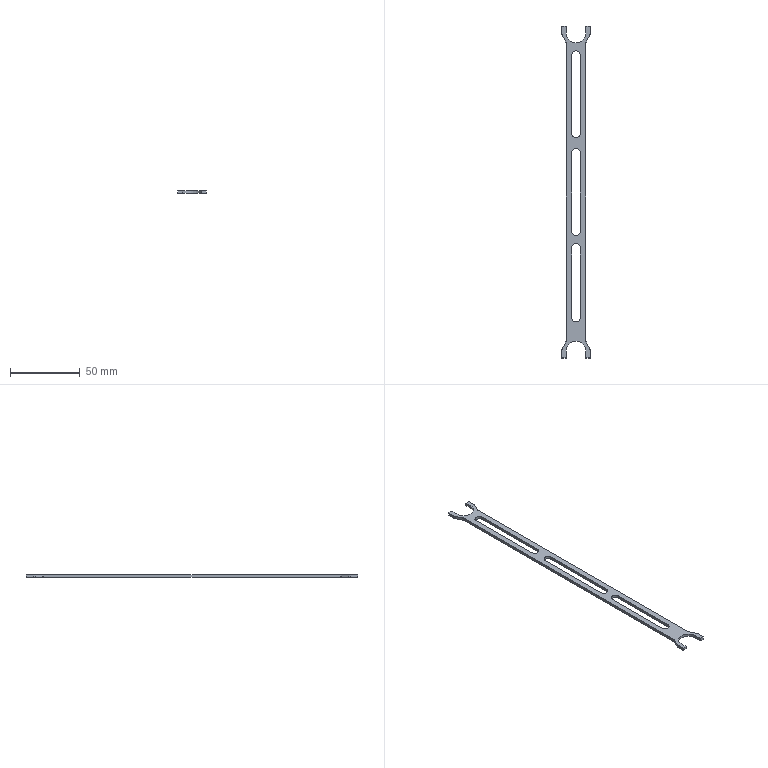Part | SolidWorks | features Extrusion 1, Fillet 1 | 1 solid | 42 faces | box 20.2 x 237.5 x 2 mm | volume 4160 mm3 | plane 26 | cylinder 16 | commonest cylinder face diameters 6 x14 14.2 x2
STEP:
#1=CARTESIAN_POINT('',(10.1,-118.75,2.));
#2=VERTEX_POINT('',#1);
#3=CARTESIAN_POINT('',(10.1,-113.469,2.));
#4=VERTEX_POINT('',#3);
#5=CARTESIAN_POINT('',(10.1,-118.75,2.));
#6=DIRECTION('',(0.,1.,0.));
#7=VECTOR('',#6,1000.);
#8=LINE('',#5,#7);
#9=EDGE_CURVE('',#2,#4,#8,.T.);
#10=ORIENTED_EDGE('',*,*,#9,.T.);
#11=CARTESIAN_POINT('',(9.774,-112.109,2.));
#12=VERTEX_POINT('',#11);
#13=CARTESIAN_POINT('',(7.1,-113.469,2.));
#14=DIRECTION('',(0.,0.,1.));
#15=DIRECTION('',(1.,0.,0.));
#16=AXIS2_PLACEMENT_3D('',#13,#14,#15);
#17=CIRCLE('',#16,3.);
#18=EDGE_CURVE('',#4,#12,#17,.T.);
#19=ORIENTED_EDGE('',*,*,#18,.T.);
#20=CARTESIAN_POINT('',(7.326,-107.291,2.));
#21=VERTEX_POINT('',#20);
#22=CARTESIAN_POINT('',(10.1,-112.75,2.));
#23=DIRECTION('',(-0.453,0.8915,0.));
#24=VECTOR('',#23,1000.);
#25=LINE('',#22,#24);
#26=EDGE_CURVE('',#12,#21,#25,.T.);
#27=ORIENTED_EDGE('',*,*,#26,.T.);
#28=CARTESIAN_POINT('',(7.,-105.931,2.));
#29=VERTEX_POINT('',#28);
#30=CARTESIAN_POINT('',(10.,-105.931,2.));
#31=DIRECTION('',(0.,0.,-1.));
#32=DIRECTION('',(1.,0.,0.));
#33=AXIS2_PLACEMENT_3D('',#30,#31,#32);
#34=CIRCLE('',#33,3.);
#35=EDGE_CURVE('',#21,#29,#34,.T.);
#36=ORIENTED_EDGE('',*,*,#35,.T.);
#37=CARTESIAN_POINT('',(7.,105.931,2.));
#38=VERTEX_POINT('',#37);
#39=CARTESIAN_POINT('',(7.,106.65,2.));
#40=DIRECTION('',(0.,1.,0.));
#41=VECTOR('',#40,1000.);
#42=LINE('',#39,#41);
#43=EDGE_CURVE('',#29,#38,#42,.T.);
#44=ORIENTED_EDGE('',*,*,#43,.T.);
#45=CARTESIAN_POINT('',(7.326,107.291,2.));
#46=VERTEX_POINT('',#45);
#47=CARTESIAN_POINT('',(10.,105.931,2.));
#48=DIRECTION('',(0.,0.,-1.));
#49=DIRECTION('',(1.,0.,0.));
#50=AXIS2_PLACEMENT_3D('',#47,#48,#49);
#51=CIRCLE('',#50,3.);
#52=EDGE_CURVE('',#38,#46,#51,.T.);
#53=ORIENTED_EDGE('',*,*,#52,.T.);
#54=CARTESIAN_POINT('',(9.774,112.109,2.));
#55=VERTEX_POINT('',#54);
#56=CARTESIAN_POINT('',(10.1,112.75,2.));
#57=DIRECTION('',(0.453,0.8915,0.));
#58=VECTOR('',#57,1000.);
#59=LINE('',#56,#58);
#60=EDGE_CURVE('',#46,#55,#59,.T.);
#61=ORIENTED_EDGE('',*,*,#60,.T.);
#62=CARTESIAN_POINT('',(10.1,113.469,2.));
#63=VERTEX_POINT('',#62);
#64=CARTESIAN_POINT('',(7.1,113.469,2.));
#65=DIRECTION('',(0.,0.,1.));
#66=DIRECTION('',(1.,0.,0.));
#67=AXIS2_PLACEMENT_3D('',#64,#65,#66);
#68=CIRCLE('',#67,3.);
#69=EDGE_CURVE('',#55,#63,#68,.T.);
#70=ORIENTED_EDGE('',*,*,#69,.T.);
#71=CARTESIAN_POINT('',(10.1,118.75,2.));
#72=VERTEX_POINT('',#71);
#73=CARTESIAN_POINT('',(10.1,118.75,2.));
#74=DIRECTION('',(0.,1.,0.));
#75=VECTOR('',#74,1000.);
#76=LINE('',#73,#75);
#77=EDGE_CURVE('',#63,#72,#76,.T.);
#78=ORIENTED_EDGE('',*,*,#77,.T.);
#79=CARTESIAN_POINT('',(7.1,118.75,2.));
#80=VERTEX_POINT('',#79);
#81=CARTESIAN_POINT('',(7.1,118.75,2.));
#82=DIRECTION('',(-1.,0.,0.));
#83=VECTOR('',#82,1000.);
#84=LINE('',#81,#83);
#85=EDGE_CURVE('',#72,#80,#84,.T.);
#86=ORIENTED_EDGE('',*,*,#85,.T.);
#87=CARTESIAN_POINT('',(7.1,113.75,2.));
#88=VERTEX_POINT('',#87);
#89=CARTESIAN_POINT('',(7.1,113.75,2.));
#90=DIRECTION('',(0.,-1.,0.));
#91=VECTOR('',#90,1000.);
#92=LINE('',#89,#91);
#93=EDGE_CURVE('',#80,#88,#92,.T.);
#94=ORIENTED_EDGE('',*,*,#93,.T.);
#95=CARTESIAN_POINT('',(-7.1,113.75,2.));
#96=VERTEX_POINT('',#95);
#97=CARTESIAN_POINT('',(0.,113.75,2.));
#98=DIRECTION('',(0.,0.,-1.));
#99=DIRECTION('',(1.,0.,0.));
#100=AXIS2_PLACEMENT_3D('',#97,#98,#99);
#101=CIRCLE('',#100,7.1);
#102=EDGE_CURVE('',#88,#96,#101,.T.);
#103=ORIENTED_EDGE('',*,*,#102,.T.);
#104=CARTESIAN_POINT('',(-7.1,118.75,2.));
#105=VERTEX_POINT('',#104);
#106=CARTESIAN_POINT('',(-7.1,113.75,2.));
#107=DIRECTION('',(0.,1.,0.));
#108=VECTOR('',#107,1000.);
#109=LINE('',#106,#108);
#110=EDGE_CURVE('',#96,#105,#109,.T.);
#111=ORIENTED_EDGE('',*,*,#110,.T.);
#112=CARTESIAN_POINT('',(-10.1,118.75,2.));
#113=VERTEX_POINT('',#112);
#114=CARTESIAN_POINT('',(-7.1,118.75,2.));
#115=DIRECTION('',(-1.,0.,0.));
#116=VECTOR('',#115,1000.);
#117=LINE('',#114,#116);
#118=EDGE_CURVE('',#105,#113,#117,.T.);
#119=ORIENTED_EDGE('',*,*,#118,.T.);
#120=CARTESIAN_POINT('',(-10.1,113.469,2.));
#121=VERTEX_POINT('',#120);
#122=CARTESIAN_POINT('',(-10.1,118.75,2.));
#123=DIRECTION('',(0.,-1.,0.));
#124=VECTOR('',#123,1000.);
#125=LINE('',#122,#124);
#126=EDGE_CURVE('',#113,#121,#125,.T.);
#127=ORIENTED_EDGE('',*,*,#126,.T.);
#128=CARTESIAN_POINT('',(-9.774,112.109,2.));
#129=VERTEX_POINT('',#128);
#130=CARTESIAN_POINT('',(-7.1,113.469,2.));
#131=DIRECTION('',(0.,0.,1.));
#132=DIRECTION('',(1.,0.,0.));
#133=AXIS2_PLACEMENT_3D('',#130,#131,#132);
#134=CIRCLE('',#133,3.);
#135=EDGE_CURVE('',#121,#129,#134,.T.);
#136=ORIENTED_EDGE('',*,*,#135,.T.);
#137=CARTESIAN_POINT('',(-7.326,107.291,2.));
#138=VERTEX_POINT('',#137);
#139=CARTESIAN_POINT('',(-10.1,112.75,2.));
#140=DIRECTION('',(0.453,-0.8915,0.));
#141=VECTOR('',#140,1000.);
#142=LINE('',#139,#141);
#143=EDGE_CURVE('',#129,#138,#142,.T.);
#144=ORIENTED_EDGE('',*,*,#143,.T.);
#145=CARTESIAN_POINT('',(-7.,105.931,2.));
#146=VERTEX_POINT('',#145);
#147=CARTESIAN_POINT('',(-10.,105.931,2.));
#148=DIRECTION('',(0.,0.,-1.));
#149=DIRECTION('',(1.,0.,0.));
#150=AXIS2_PLACEMENT_3D('',#147,#148,#149);
#151=CIRCLE('',#150,3.);
#152=EDGE_CURVE('',#138,#146,#151,.T.);
#153=ORIENTED_EDGE('',*,*,#152,.T.);
#154=CARTESIAN_POINT('',(-7.,-105.931,2.));
#155=VERTEX_POINT('',#154);
#156=CARTESIAN_POINT('',(-7.,106.65,2.));
#157=DIRECTION('',(0.,-1.,0.));
#158=VECTOR('',#157,1000.);
#159=LINE('',#156,#158);
#160=EDGE_CURVE('',#146,#155,#159,.T.);
#161=ORIENTED_EDGE('',*,*,#160,.T.);
#162=CARTESIAN_POINT('',(-7.326,-107.291,2.));
#163=VERTEX_POINT('',#162);
#164=CARTESIAN_POINT('',(-10.,-105.931,2.));
#165=DIRECTION('',(0.,0.,-1.));
#166=DIRECTION('',(1.,0.,0.));
#167=AXIS2_PLACEMENT_3D('',#164,#165,#166);
#168=CIRCLE('',#167,3.);
#169=EDGE_CURVE('',#155,#163,#168,.T.);
#170=ORIENTED_EDGE('',*,*,#169,.T.);
#171=CARTESIAN_POINT('',(-9.774,-112.109,2.));
#172=VERTEX_POINT('',#171);
#173=CARTESIAN_POINT('',(-10.1,-112.75,2.));
#174=DIRECTION('',(-0.453,-0.8915,0.));
#175=VECTOR('',#174,1000.);
#176=LINE('',#173,#175);
#177=EDGE_CURVE('',#163,#172,#176,.T.);
#178=ORIENTED_EDGE('',*,*,#177,.T.);
#179=CARTESIAN_POINT('',(-10.1,-113.469,2.));
#180=VERTEX_POINT('',#179);
#181=CARTESIAN_POINT('',(-7.1,-113.469,2.));
#182=DIRECTION('',(0.,0.,1.));
#183=DIRECTION('',(1.,0.,0.));
#184=AXIS2_PLACEMENT_3D('',#181,#182,#183);
#185=CIRCLE('',#184,3.);
#186=EDGE_CURVE('',#172,#180,#185,.T.);
#187=ORIENTED_EDGE('',*,*,#186,.T.);
#188=CARTESIAN_POINT('',(-10.1,-118.75,2.));
#189=VERTEX_POINT('',#188);
#190=CARTESIAN_POINT('',(-10.1,-118.75,2.));
#191=DIRECTION('',(0.,-1.,0.));
#192=VECTOR('',#191,1000.);
#193=LINE('',#190,#192);
#194=EDGE_CURVE('',#180,#189,#193,.T.);
#195=ORIENTED_EDGE('',*,*,#194,.T.);
#196=CARTESIAN_POINT('',(-7.1,-118.75,2.));
#197=VERTEX_POINT('',#196);
#198=CARTESIAN_POINT('',(-7.1,-118.75,2.));
#199=DIRECTION('',(1.,0.,0.));
#200=VECTOR('',#199,1000.);
#201=LINE('',#198,#200);
#202=EDGE_CURVE('',#189,#197,#201,.T.);
#203=ORIENTED_EDGE('',*,*,#202,.T.);
#204=CARTESIAN_POINT('',(-7.1,-113.75,2.));
#205=VERTEX_POINT('',#204);
#206=CARTESIAN_POINT('',(-7.1,-113.75,2.));
#207=DIRECTION('',(0.,1.,0.));
#208=VECTOR('',#207,1000.);
#209=LINE('',#206,#208);
#210=EDGE_CURVE('',#197,#205,#209,.T.);
#211=ORIENTED_EDGE('',*,*,#210,.T.);
#212=CARTESIAN_POINT('',(7.1,-113.75,2.));
#213=VERTEX_POINT('',#212);
#214=CARTESIAN_POINT('',(0.,-113.75,2.));
#215=DIRECTION('',(0.,0.,-1.));
#216=DIRECTION('',(1.,0.,0.));
#217=AXIS2_PLACEMENT_3D('',#214,#215,#216);
#218=CIRCLE('',#217,7.1);
#219=EDGE_CURVE('',#205,#213,#218,.T.);
#220=ORIENTED_EDGE('',*,*,#219,.T.);
#221=CARTESIAN_POINT('',(7.1,-118.75,2.));
#222=VERTEX_POINT('',#221);
#223=CARTESIAN_POINT('',(7.1,-113.75,2.));
#224=DIRECTION('',(0.,-1.,0.));
#225=VECTOR('',#224,1000.);
#226=LINE('',#223,#225);
#227=EDGE_CURVE('',#213,#222,#226,.T.);
#228=ORIENTED_EDGE('',*,*,#227,.T.);
#229=CARTESIAN_POINT('',(7.1,-118.75,2.));
#230=DIRECTION('',(1.,0.,0.));
#231=VECTOR('',#230,1000.);
#232=LINE('',#229,#231);
#233=EDGE_CURVE('',#222,#2,#232,.T.);
#234=ORIENTED_EDGE('',*,*,#233,.T.);
#235=EDGE_LOOP('',(#10,#19,#27,#36,#44,#53,#61,#70,#78,#86,#94,#103,#111,#119,#127,#136,#144,#153,#161,#170,#178,#187,#195,#203,#211,#220,#228,#234));
#236=FACE_OUTER_BOUND('',#235,.T.);
#237=CARTESIAN_POINT('',(-3.,98.,2.));
#238=VERTEX_POINT('',#237);
#239=CARTESIAN_POINT('',(-3.,42.,2.));
#240=VERTEX_POINT('',#239);
#241=CARTESIAN_POINT('',(-3.,98.,2.));
#242=DIRECTION('',(0.,-1.,0.));
#243=VECTOR('',#242,1000.);
#244=LINE('',#241,#243);
#245=EDGE_CURVE('',#238,#240,#244,.T.);
#246=ORIENTED_EDGE('',*,*,#245,.F.);
#247=CARTESIAN_POINT('',(3.,98.,2.));
#248=VERTEX_POINT('',#247);
#249=CARTESIAN_POINT('',(0.,98.,2.));
#250=DIRECTION('',(0.,0.,1.));
#251=DIRECTION('',(1.,0.,0.));
#252=AXIS2_PLACEMENT_3D('',#249,#250,#251);
#253=CIRCLE('',#252,3.);
#254=EDGE_CURVE('',#248,#238,#253,.T.);
#255=ORIENTED_EDGE('',*,*,#254,.F.);
#256=CARTESIAN_POINT('',(3.,42.,2.));
#257=VERTEX_POINT('',#256);
#258=CARTESIAN_POINT('',(3.,98.,2.));
#259=DIRECTION('',(0.,1.,0.));
#260=VECTOR('',#259,1000.);
#261=LINE('',#258,#260);
#262=EDGE_CURVE('',#257,#248,#261,.T.);
#263=ORIENTED_EDGE('',*,*,#262,.F.);
#264=CARTESIAN_POINT('',(0.,42.,2.));
#265=DIRECTION('',(0.,0.,1.));
#266=DIRECTION('',(1.,0.,0.));
#267=AXIS2_PLACEMENT_3D('',#264,#265,#266);
#268=CIRCLE('',#267,3.);
#269=EDGE_CURVE('',#240,#257,#268,.T.);
#270=ORIENTED_EDGE('',*,*,#269,.F.);
#271=EDGE_LOOP('',(#246,#255,#263,#270));
#272=FACE_BOUND('',#271,.T.);
#273=CARTESIAN_POINT('',(-3.,28.,2.));
#274=VERTEX_POINT('',#273);
#275=CARTESIAN_POINT('',(-3.,-28.,2.));
#276=VERTEX_POINT('',#275);
#277=CARTESIAN_POINT('',(-3.,28.,2.));
#278=DIRECTION('',(0.,-1.,0.));
#279=VECTOR('',#278,1000.);
#280=LINE('',#277,#279);
#281=EDGE_CURVE('',#274,#276,#280,.T.);
#282=ORIENTED_EDGE('',*,*,#281,.F.);
#283=CARTESIAN_POINT('',(3.,28.,2.));
#284=VERTEX_POINT('',#283);
#285=CARTESIAN_POINT('',(0.,28.,2.));
#286=DIRECTION('',(0.,0.,1.));
#287=DIRECTION('',(1.,0.,0.));
#288=AXIS2_PLACEMENT_3D('',#285,#286,#287);
#289=CIRCLE('',#288,3.);
#290=EDGE_CURVE('',#284,#274,#289,.T.);
#291=ORIENTED_EDGE('',*,*,#290,.F.);
#292=CARTESIAN_POINT('',(3.,-28.,2.));
#293=VERTEX_POINT('',#292);
#294=CARTESIAN_POINT('',(3.,28.,2.));
#295=DIRECTION('',(0.,1.,0.));
#296=VECTOR('',#295,1000.);
#297=LINE('',#294,#296);
#298=EDGE_CURVE('',#293,#284,#297,.T.);
#299=ORIENTED_EDGE('',*,*,#298,.F.);
#300=CARTESIAN_POINT('',(0.,-28.,2.));
#301=DIRECTION('',(0.,0.,1.));
#302=DIRECTION('',(1.,0.,0.));
#303=AXIS2_PLACEMENT_3D('',#300,#301,#302);
#304=CIRCLE('',#303,3.);
#305=EDGE_CURVE('',#276,#293,#304,.T.);
#306=ORIENTED_EDGE('',*,*,#305,.F.);
#307=EDGE_LOOP('',(#282,#291,#299,#306));
#308=FACE_BOUND('',#307,.T.);
#309=CARTESIAN_POINT('',(-3.,-40.,2.));
#310=VERTEX_POINT('',#309);
#311=CARTESIAN_POINT('',(-3.,-90.,2.));
#312=VERTEX_POINT('',#311);
#313=CARTESIAN_POINT('',(-3.,-40.,2.));
#314=DIRECTION('',(0.,-1.,0.));
#315=VECTOR('',#314,1000.);
#316=LINE('',#313,#315);
#317=EDGE_CURVE('',#310,#312,#316,.T.);
#318=ORIENTED_EDGE('',*,*,#317,.F.);
#319=CARTESIAN_POINT('',(3.,-40.,2.));
#320=VERTEX_POINT('',#319);
#321=CARTESIAN_POINT('',(0.,-40.,2.));
#322=DIRECTION('',(0.,0.,1.));
#323=DIRECTION('',(1.,0.,0.));
#324=AXIS2_PLACEMENT_3D('',#321,#322,#323);
#325=CIRCLE('',#324,3.);
#326=EDGE_CURVE('',#320,#310,#325,.T.);
#327=ORIENTED_EDGE('',*,*,#326,.F.);
#328=CARTESIAN_POINT('',(3.,-90.,2.));
#329=VERTEX_POINT('',#328);
#330=CARTESIAN_POINT('',(3.,-40.,2.));
#331=DIRECTION('',(0.,1.,0.));
#332=VECTOR('',#331,1000.);
#333=LINE('',#330,#332);
#334=EDGE_CURVE('',#329,#320,#333,.T.);
#335=ORIENTED_EDGE('',*,*,#334,.F.);
#336=CARTESIAN_POINT('',(0.,-90.,2.));
#337=DIRECTION('',(0.,0.,1.));
#338=DIRECTION('',(1.,0.,0.));
#339=AXIS2_PLACEMENT_3D('',#336,#337,#338);
#340=CIRCLE('',#339,3.);
#341=EDGE_CURVE('',#312,#329,#340,.T.);
#342=ORIENTED_EDGE('',*,*,#341,.F.);
#343=EDGE_LOOP('',(#318,#327,#335,#342));
#344=FACE_BOUND('',#343,.T.);
#345=CARTESIAN_POINT('',(0.,113.75,2.));
#346=DIRECTION('',(0.,0.,1.));
#347=DIRECTION('',(1.,0.,0.));
#348=AXIS2_PLACEMENT_3D('',#345,#346,#347);
#349=PLANE('',#348);
#350=ADVANCED_FACE('',(#236,#272,#308,#344),#349,.T.);
#351=CARTESIAN_POINT('',(3.,28.,0.));
#352=VERTEX_POINT('',#351);
#353=CARTESIAN_POINT('',(-3.,28.,0.));
#354=VERTEX_POINT('',#353);
#355=CARTESIAN_POINT('',(0.,28.,0.));
#356=DIRECTION('',(0.,0.,1.));
#357=DIRECTION('',(1.,0.,0.));
#358=AXIS2_PLACEMENT_3D('',#355,#356,#357);
#359=CIRCLE('',#358,3.);
#360=EDGE_CURVE('',#352,#354,#359,.T.);
#361=ORIENTED_EDGE('',*,*,#360,.T.);
#362=CARTESIAN_POINT('',(-3.,-28.,0.));
#363=VERTEX_POINT('',#362);
#364=CARTESIAN_POINT('',(-3.,28.,0.));
#365=DIRECTION('',(0.,-1.,0.));
#366=VECTOR('',#365,1000.);
#367=LINE('',#364,#366);
#368=EDGE_CURVE('',#354,#363,#367,.T.);
#369=ORIENTED_EDGE('',*,*,#368,.T.);
#370=CARTESIAN_POINT('',(3.,-28.,0.));
#371=VERTEX_POINT('',#370);
#372=CARTESIAN_POINT('',(0.,-28.,0.));
#373=DIRECTION('',(0.,0.,1.));
#374=DIRECTION('',(1.,0.,0.));
#375=AXIS2_PLACEMENT_3D('',#372,#373,#374);
#376=CIRCLE('',#375,3.);
#377=EDGE_CURVE('',#363,#371,#376,.T.);
#378=ORIENTED_EDGE('',*,*,#377,.T.);
#379=CARTESIAN_POINT('',(3.,28.,0.));
#380=DIRECTION('',(0.,1.,0.));
#381=VECTOR('',#380,1000.);
#382=LINE('',#379,#381);
#383=EDGE_CURVE('',#371,#352,#382,.T.);
#384=ORIENTED_EDGE('',*,*,#383,.T.);
#385=EDGE_LOOP('',(#361,#369,#378,#384));
#386=FACE_BOUND('',#385,.T.);
#387=CARTESIAN_POINT('',(9.774,-112.109,0.));
#388=VERTEX_POINT('',#387);
#389=CARTESIAN_POINT('',(7.326,-107.291,0.));
#390=VERTEX_POINT('',#389);
#391=CARTESIAN_POINT('',(10.1,-112.75,0.));
#392=DIRECTION('',(-0.453,0.8915,0.));
#393=VECTOR('',#392,1000.);
#394=LINE('',#391,#393);
#395=EDGE_CURVE('',#388,#390,#394,.T.);
#396=ORIENTED_EDGE('',*,*,#395,.F.);
#397=CARTESIAN_POINT('',(10.1,-113.469,0.));
#398=VERTEX_POINT('',#397);
#399=CARTESIAN_POINT('',(7.1,-113.469,0.));
#400=DIRECTION('',(0.,0.,-1.));
#401=DIRECTION('',(1.,0.,0.));
#402=AXIS2_PLACEMENT_3D('',#399,#400,#401);
#403=CIRCLE('',#402,3.);
#404=EDGE_CURVE('',#388,#398,#403,.T.);
#405=ORIENTED_EDGE('',*,*,#404,.T.);
#406=CARTESIAN_POINT('',(10.1,-118.75,0.));
#407=VERTEX_POINT('',#406);
#408=CARTESIAN_POINT('',(10.1,-118.75,0.));
#409=DIRECTION('',(0.,1.,0.));
#410=VECTOR('',#409,1000.);
#411=LINE('',#408,#410);
#412=EDGE_CURVE('',#407,#398,#411,.T.);
#413=ORIENTED_EDGE('',*,*,#412,.F.);
#414=CARTESIAN_POINT('',(7.1,-118.75,0.));
#415=VERTEX_POINT('',#414);
#416=CARTESIAN_POINT('',(7.1,-118.75,0.));
#417=DIRECTION('',(1.,0.,0.));
#418=VECTOR('',#417,1000.);
#419=LINE('',#416,#418);
#420=EDGE_CURVE('',#415,#407,#419,.T.);
#421=ORIENTED_EDGE('',*,*,#420,.F.);
#422=CARTESIAN_POINT('',(7.1,-113.75,0.));
#423=VERTEX_POINT('',#422);
#424=CARTESIAN_POINT('',(7.1,-113.75,0.));
#425=DIRECTION('',(0.,-1.,0.));
#426=VECTOR('',#425,1000.);
#427=LINE('',#424,#426);
#428=EDGE_CURVE('',#423,#415,#427,.T.);
#429=ORIENTED_EDGE('',*,*,#428,.F.);
#430=CARTESIAN_POINT('',(-7.1,-113.75,0.));
#431=VERTEX_POINT('',#430);
#432=CARTESIAN_POINT('',(0.,-113.75,0.));
#433=DIRECTION('',(0.,0.,-1.));
#434=DIRECTION('',(1.,0.,0.));
#435=AXIS2_PLACEMENT_3D('',#432,#433,#434);
#436=CIRCLE('',#435,7.1);
#437=EDGE_CURVE('',#431,#423,#436,.T.);
#438=ORIENTED_EDGE('',*,*,#437,.F.);
#439=CARTESIAN_POINT('',(-7.1,-118.75,0.));
#440=VERTEX_POINT('',#439);
#441=CARTESIAN_POINT('',(-7.1,-113.75,0.));
#442=DIRECTION('',(0.,1.,0.));
#443=VECTOR('',#442,1000.);
#444=LINE('',#441,#443);
#445=EDGE_CURVE('',#440,#431,#444,.T.);
#446=ORIENTED_EDGE('',*,*,#445,.F.);
#447=CARTESIAN_POINT('',(-10.1,-118.75,0.));
#448=VERTEX_POINT('',#447);
#449=CARTESIAN_POINT('',(-7.1,-118.75,0.));
#450=DIRECTION('',(1.,0.,0.));
#451=VECTOR('',#450,1000.);
#452=LINE('',#449,#451);
#453=EDGE_CURVE('',#448,#440,#452,.T.);
#454=ORIENTED_EDGE('',*,*,#453,.F.);
#455=CARTESIAN_POINT('',(-10.1,-113.469,0.));
#456=VERTEX_POINT('',#455);
#457=CARTESIAN_POINT('',(-10.1,-118.75,0.));
#458=DIRECTION('',(0.,-1.,0.));
#459=VECTOR('',#458,1000.);
#460=LINE('',#457,#459);
#461=EDGE_CURVE('',#456,#448,#460,.T.);
#462=ORIENTED_EDGE('',*,*,#461,.F.);
#463=CARTESIAN_POINT('',(-9.774,-112.109,0.));
#464=VERTEX_POINT('',#463);
#465=CARTESIAN_POINT('',(-7.1,-113.469,0.));
#466=DIRECTION('',(0.,0.,-1.));
#467=DIRECTION('',(1.,0.,0.));
#468=AXIS2_PLACEMENT_3D('',#465,#466,#467);
#469=CIRCLE('',#468,3.);
#470=EDGE_CURVE('',#456,#464,#469,.T.);
#471=ORIENTED_EDGE('',*,*,#470,.T.);
#472=CARTESIAN_POINT('',(-7.326,-107.291,0.));
#473=VERTEX_POINT('',#472);
#474=CARTESIAN_POINT('',(-10.1,-112.75,0.));
#475=DIRECTION('',(-0.453,-0.8915,0.));
#476=VECTOR('',#475,1000.);
#477=LINE('',#474,#476);
#478=EDGE_CURVE('',#473,#464,#477,.T.);
#479=ORIENTED_EDGE('',*,*,#478,.F.);
#480=CARTESIAN_POINT('',(-7.,-105.931,0.));
#481=VERTEX_POINT('',#480);
#482=CARTESIAN_POINT('',(-10.,-105.931,0.));
#483=DIRECTION('',(0.,0.,1.));
#484=DIRECTION('',(1.,0.,0.));
#485=AXIS2_PLACEMENT_3D('',#482,#483,#484);
#486=CIRCLE('',#485,3.);
#487=EDGE_CURVE('',#473,#481,#486,.T.);
#488=ORIENTED_EDGE('',*,*,#487,.T.);
#489=CARTESIAN_POINT('',(-7.,105.931,0.));
#490=VERTEX_POINT('',#489);
#491=CARTESIAN_POINT('',(-7.,106.65,0.));
#492=DIRECTION('',(0.,-1.,0.));
#493=VECTOR('',#492,1000.);
#494=LINE('',#491,#493);
#495=EDGE_CURVE('',#490,#481,#494,.T.);
#496=ORIENTED_EDGE('',*,*,#495,.F.);
#497=CARTESIAN_POINT('',(-7.326,107.291,0.));
#498=VERTEX_POINT('',#497);
#499=CARTESIAN_POINT('',(-10.,105.931,0.));
#500=DIRECTION('',(0.,0.,1.));
#501=DIRECTION('',(1.,0.,0.));
#502=AXIS2_PLACEMENT_3D('',#499,#500,#501);
#503=CIRCLE('',#502,3.);
#504=EDGE_CURVE('',#490,#498,#503,.T.);
#505=ORIENTED_EDGE('',*,*,#504,.T.);
#506=CARTESIAN_POINT('',(-9.774,112.109,0.));
#507=VERTEX_POINT('',#506);
#508=CARTESIAN_POINT('',(-10.1,112.75,0.));
#509=DIRECTION('',(0.453,-0.8915,0.));
#510=VECTOR('',#509,1000.);
#511=LINE('',#508,#510);
#512=EDGE_CURVE('',#507,#498,#511,.T.);
#513=ORIENTED_EDGE('',*,*,#512,.F.);
#514=CARTESIAN_POINT('',(-10.1,113.469,0.));
#515=VERTEX_POINT('',#514);
#516=CARTESIAN_POINT('',(-7.1,113.469,0.));
#517=DIRECTION('',(0.,0.,-1.));
#518=DIRECTION('',(1.,0.,0.));
#519=AXIS2_PLACEMENT_3D('',#516,#517,#518);
#520=CIRCLE('',#519,3.);
#521=EDGE_CURVE('',#507,#515,#520,.T.);
#522=ORIENTED_EDGE('',*,*,#521,.T.);
#523=CARTESIAN_POINT('',(-10.1,118.75,0.));
#524=VERTEX_POINT('',#523);
#525=CARTESIAN_POINT('',(-10.1,118.75,0.));
#526=DIRECTION('',(0.,-1.,0.));
#527=VECTOR('',#526,1000.);
#528=LINE('',#525,#527);
#529=EDGE_CURVE('',#524,#515,#528,.T.);
#530=ORIENTED_EDGE('',*,*,#529,.F.);
#531=CARTESIAN_POINT('',(-7.1,118.75,0.));
#532=VERTEX_POINT('',#531);
#533=CARTESIAN_POINT('',(-7.1,118.75,0.));
#534=DIRECTION('',(-1.,0.,0.));
#535=VECTOR('',#534,1000.);
#536=LINE('',#533,#535);
#537=EDGE_CURVE('',#532,#524,#536,.T.);
#538=ORIENTED_EDGE('',*,*,#537,.F.);
#539=CARTESIAN_POINT('',(-7.1,113.75,0.));
#540=VERTEX_POINT('',#539);
#541=CARTESIAN_POINT('',(-7.1,113.75,0.));
#542=DIRECTION('',(0.,1.,0.));
#543=VECTOR('',#542,1000.);
#544=LINE('',#541,#543);
#545=EDGE_CURVE('',#540,#532,#544,.T.);
#546=ORIENTED_EDGE('',*,*,#545,.F.);
#547=CARTESIAN_POINT('',(7.1,113.75,0.));
#548=VERTEX_POINT('',#547);
#549=CARTESIAN_POINT('',(0.,113.75,0.));
#550=DIRECTION('',(0.,0.,-1.));
#551=DIRECTION('',(1.,0.,0.));
#552=AXIS2_PLACEMENT_3D('',#549,#550,#551);
#553=CIRCLE('',#552,7.1);
#554=EDGE_CURVE('',#548,#540,#553,.T.);
#555=ORIENTED_EDGE('',*,*,#554,.F.);
#556=CARTESIAN_POINT('',(7.1,118.75,0.));
#557=VERTEX_POINT('',#556);
#558=CARTESIAN_POINT('',(7.1,113.75,0.));
#559=DIRECTION('',(0.,-1.,0.));
#560=VECTOR('',#559,1000.);
#561=LINE('',#558,#560);
#562=EDGE_CURVE('',#557,#548,#561,.T.);
#563=ORIENTED_EDGE('',*,*,#562,.F.);
#564=CARTESIAN_POINT('',(10.1,118.75,0.));
#565=VERTEX_POINT('',#564);
#566=CARTESIAN_POINT('',(7.1,118.75,0.));
#567=DIRECTION('',(-1.,0.,0.));
#568=VECTOR('',#567,1000.);
#569=LINE('',#566,#568);
#570=EDGE_CURVE('',#565,#557,#569,.T.);
#571=ORIENTED_EDGE('',*,*,#570,.F.);
#572=CARTESIAN_POINT('',(10.1,113.469,0.));
#573=VERTEX_POINT('',#572);
#574=CARTESIAN_POINT('',(10.1,118.75,0.));
#575=DIRECTION('',(0.,1.,0.));
#576=VECTOR('',#575,1000.);
#577=LINE('',#574,#576);
#578=EDGE_CURVE('',#573,#565,#577,.T.);
#579=ORIENTED_EDGE('',*,*,#578,.F.);
#580=CARTESIAN_POINT('',(9.774,112.109,0.));
#581=VERTEX_POINT('',#580);
#582=CARTESIAN_POINT('',(7.1,113.469,0.));
#583=DIRECTION('',(0.,0.,-1.));
#584=DIRECTION('',(1.,0.,0.));
#585=AXIS2_PLACEMENT_3D('',#582,#583,#584);
#586=CIRCLE('',#585,3.);
#587=EDGE_CURVE('',#573,#581,#586,.T.);
#588=ORIENTED_EDGE('',*,*,#587,.T.);
#589=CARTESIAN_POINT('',(7.326,107.291,0.));
#590=VERTEX_POINT('',#589);
#591=CARTESIAN_POINT('',(10.1,112.75,0.));
#592=DIRECTION('',(0.453,0.8915,0.));
#593=VECTOR('',#592,1000.);
#594=LINE('',#591,#593);
#595=EDGE_CURVE('',#590,#581,#594,.T.);
#596=ORIENTED_EDGE('',*,*,#595,.F.);
#597=CARTESIAN_POINT('',(7.,105.931,0.));
#598=VERTEX_POINT('',#597);
#599=CARTESIAN_POINT('',(10.,105.931,0.));
#600=DIRECTION('',(0.,0.,1.));
#601=DIRECTION('',(1.,0.,0.));
#602=AXIS2_PLACEMENT_3D('',#599,#600,#601);
#603=CIRCLE('',#602,3.);
#604=EDGE_CURVE('',#590,#598,#603,.T.);
#605=ORIENTED_EDGE('',*,*,#604,.T.);
#606=CARTESIAN_POINT('',(7.,-105.931,0.));
#607=VERTEX_POINT('',#606);
#608=CARTESIAN_POINT('',(7.,106.65,0.));
#609=DIRECTION('',(0.,1.,0.));
#610=VECTOR('',#609,1000.);
#611=LINE('',#608,#610);
#612=EDGE_CURVE('',#607,#598,#611,.T.);
#613=ORIENTED_EDGE('',*,*,#612,.F.);
#614=CARTESIAN_POINT('',(10.,-105.931,0.));
#615=DIRECTION('',(0.,0.,1.));
#616=DIRECTION('',(1.,0.,0.));
#617=AXIS2_PLACEMENT_3D('',#614,#615,#616);
#618=CIRCLE('',#617,3.);
#619=EDGE_CURVE('',#607,#390,#618,.T.);
#620=ORIENTED_EDGE('',*,*,#619,.T.);
#621=EDGE_LOOP('',(#396,#405,#413,#421,#429,#438,#446,#454,#462,#471,#479,#488,#496,#505,#513,#522,#530,#538,#546,#555,#563,#571,#579,#588,#596,#605,#613,#620));
#622=FACE_OUTER_BOUND('',#621,.T.);
#623=CARTESIAN_POINT('',(3.,98.,0.));
#624=VERTEX_POINT('',#623);
#625=CARTESIAN_POINT('',(-3.,98.,0.));
#626=VERTEX_POINT('',#625);
#627=CARTESIAN_POINT('',(0.,98.,0.));
#628=DIRECTION('',(0.,0.,1.));
#629=DIRECTION('',(1.,0.,0.));
#630=AXIS2_PLACEMENT_3D('',#627,#628,#629);
#631=CIRCLE('',#630,3.);
#632=EDGE_CURVE('',#624,#626,#631,.T.);
#633=ORIENTED_EDGE('',*,*,#632,.T.);
#634=CARTESIAN_POINT('',(-3.,42.,0.));
#635=VERTEX_POINT('',#634);
#636=CARTESIAN_POINT('',(-3.,98.,0.));
#637=DIRECTION('',(0.,-1.,0.));
#638=VECTOR('',#637,1000.);
#639=LINE('',#636,#638);
#640=EDGE_CURVE('',#626,#635,#639,.T.);
#641=ORIENTED_EDGE('',*,*,#640,.T.);
#642=CARTESIAN_POINT('',(3.,42.,0.));
#643=VERTEX_POINT('',#642);
#644=CARTESIAN_POINT('',(0.,42.,0.));
#645=DIRECTION('',(0.,0.,1.));
#646=DIRECTION('',(1.,0.,0.));
#647=AXIS2_PLACEMENT_3D('',#644,#645,#646);
#648=CIRCLE('',#647,3.);
#649=EDGE_CURVE('',#635,#643,#648,.T.);
#650=ORIENTED_EDGE('',*,*,#649,.T.);
#651=CARTESIAN_POINT('',(3.,98.,0.));
#652=DIRECTION('',(0.,1.,0.));
#653=VECTOR('',#652,1000.);
#654=LINE('',#651,#653);
#655=EDGE_CURVE('',#643,#624,#654,.T.);
#656=ORIENTED_EDGE('',*,*,#655,.T.);
#657=EDGE_LOOP('',(#633,#641,#650,#656));
#658=FACE_BOUND('',#657,.T.);
#659=CARTESIAN_POINT('',(3.,-40.,0.));
#660=VERTEX_POINT('',#659);
#661=CARTESIAN_POINT('',(-3.,-40.,0.));
#662=VERTEX_POINT('',#661);
#663=CARTESIAN_POINT('',(0.,-40.,0.));
#664=DIRECTION('',(0.,0.,1.));
#665=DIRECTION('',(1.,0.,0.));
#666=AXIS2_PLACEMENT_3D('',#663,#664,#665);
#667=CIRCLE('',#666,3.);
#668=EDGE_CURVE('',#660,#662,#667,.T.);
#669=ORIENTED_EDGE('',*,*,#668,.T.);
#670=CARTESIAN_POINT('',(-3.,-90.,0.));
#671=VERTEX_POINT('',#670);
#672=CARTESIAN_POINT('',(-3.,-40.,0.));
#673=DIRECTION('',(0.,-1.,0.));
#674=VECTOR('',#673,1000.);
#675=LINE('',#672,#674);
#676=EDGE_CURVE('',#662,#671,#675,.T.);
#677=ORIENTED_EDGE('',*,*,#676,.T.);
#678=CARTESIAN_POINT('',(3.,-90.,0.));
#679=VERTEX_POINT('',#678);
#680=CARTESIAN_POINT('',(0.,-90.,0.));
#681=DIRECTION('',(0.,0.,1.));
#682=DIRECTION('',(1.,0.,0.));
#683=AXIS2_PLACEMENT_3D('',#680,#681,#682);
#684=CIRCLE('',#683,3.);
#685=EDGE_CURVE('',#671,#679,#684,.T.);
#686=ORIENTED_EDGE('',*,*,#685,.T.);
#687=CARTESIAN_POINT('',(3.,-40.,0.));
#688=DIRECTION('',(0.,1.,0.));
#689=VECTOR('',#688,1000.);
#690=LINE('',#687,#689);
#691=EDGE_CURVE('',#679,#660,#690,.T.);
#692=ORIENTED_EDGE('',*,*,#691,.T.);
#693=EDGE_LOOP('',(#669,#677,#686,#692));
#694=FACE_BOUND('',#693,.T.);
#695=CARTESIAN_POINT('',(0.,113.75,0.));
#696=DIRECTION('',(0.,0.,1.));
#697=DIRECTION('',(1.,0.,0.));
#698=AXIS2_PLACEMENT_3D('',#695,#696,#697);
#699=PLANE('',#698);
#700=ADVANCED_FACE('',(#386,#622,#658,#694),#699,.F.);
#701=ORIENTED_EDGE('',*,*,#554,.T.);
#702=CARTESIAN_POINT('',(-7.1,113.75,2.));
#703=DIRECTION('',(0.,0.,-1.));
#704=VECTOR('',#703,1000.);
#705=LINE('',#702,#704);
#706=EDGE_CURVE('',#96,#540,#705,.T.);
#707=ORIENTED_EDGE('',*,*,#706,.F.);
#708=ORIENTED_EDGE('',*,*,#102,.F.);
#709=CARTESIAN_POINT('',(7.1,113.75,2.));
#710=DIRECTION('',(0.,0.,-1.));
#711=VECTOR('',#710,1000.);
#712=LINE('',#709,#711);
#713=EDGE_CURVE('',#88,#548,#712,.T.);
#714=ORIENTED_EDGE('',*,*,#713,.T.);
#715=EDGE_LOOP('',(#701,#707,#708,#714));
#716=FACE_OUTER_BOUND('',#715,.T.);
#717=CARTESIAN_POINT('',(0.,113.75,2.));
#718=DIRECTION('',(0.,0.,-1.));
#719=DIRECTION('',(-1.,0.,0.));
#720=AXIS2_PLACEMENT_3D('',#717,#718,#719);
#721=CYLINDRICAL_SURFACE('',#720,7.1);
#722=ADVANCED_FACE('',(#716),#721,.F.);
#723=ORIENTED_EDGE('',*,*,#545,.T.);
#724=CARTESIAN_POINT('',(-7.1,118.75,2.));
#725=DIRECTION('',(0.,0.,-1.));
#726=VECTOR('',#725,1000.);
#727=LINE('',#724,#726);
#728=EDGE_CURVE('',#105,#532,#727,.T.);
#729=ORIENTED_EDGE('',*,*,#728,.F.);
#730=ORIENTED_EDGE('',*,*,#110,.F.);
#731=ORIENTED_EDGE('',*,*,#706,.T.);
#732=EDGE_LOOP('',(#723,#729,#730,#731));
#733=FACE_OUTER_BOUND('',#732,.T.);
#734=CARTESIAN_POINT('',(-7.1,113.75,2.));
#735=DIRECTION('',(-1.,0.,0.));
#736=DIRECTION('',(0.,-1.,0.));
#737=AXIS2_PLACEMENT_3D('',#734,#735,#736);
#738=PLANE('',#737);
#739=ADVANCED_FACE('',(#733),#738,.F.);
#740=ORIENTED_EDGE('',*,*,#537,.T.);
#741=CARTESIAN_POINT('',(-10.1,118.75,2.));
#742=DIRECTION('',(0.,0.,-1.));
#743=VECTOR('',#742,1000.);
#744=LINE('',#741,#743);
#745=EDGE_CURVE('',#113,#524,#744,.T.);
#746=ORIENTED_EDGE('',*,*,#745,.F.);
#747=ORIENTED_EDGE('',*,*,#118,.F.);
#748=ORIENTED_EDGE('',*,*,#728,.T.);
#749=EDGE_LOOP('',(#740,#746,#747,#748));
#750=FACE_OUTER_BOUND('',#749,.T.);
#751=CARTESIAN_POINT('',(-7.1,118.75,2.));
#752=DIRECTION('',(0.,-1.,0.));
#753=DIRECTION('',(0.,0.,-1.));
#754=AXIS2_PLACEMENT_3D('',#751,#752,#753);
#755=PLANE('',#754);
#756=ADVANCED_FACE('',(#750),#755,.F.);
#757=ORIENTED_EDGE('',*,*,#529,.T.);
#758=CARTESIAN_POINT('',(-10.1,113.469,2.));
#759=DIRECTION('',(0.,0.,1.));
#760=VECTOR('',#759,1000.);
#761=LINE('',#758,#760);
#762=EDGE_CURVE('',#515,#121,#761,.T.);
#763=ORIENTED_EDGE('',*,*,#762,.T.);
#764=ORIENTED_EDGE('',*,*,#126,.F.);
#765=ORIENTED_EDGE('',*,*,#745,.T.);
#766=EDGE_LOOP('',(#757,#763,#764,#765));
#767=FACE_OUTER_BOUND('',#766,.T.);
#768=CARTESIAN_POINT('',(-10.1,118.75,2.));
#769=DIRECTION('',(1.,0.,0.));
#770=DIRECTION('',(0.,1.,0.));
#771=AXIS2_PLACEMENT_3D('',#768,#769,#770);
#772=PLANE('',#771);
#773=ADVANCED_FACE('',(#767),#772,.F.);
#774=ORIENTED_EDGE('',*,*,#512,.T.);
#775=CARTESIAN_POINT('',(-7.326,107.291,2.));
#776=DIRECTION('',(0.,0.,1.));
#777=VECTOR('',#776,1000.);
#778=LINE('',#775,#777);
#779=EDGE_CURVE('',#498,#138,#778,.T.);
#780=ORIENTED_EDGE('',*,*,#779,.T.);
#781=ORIENTED_EDGE('',*,*,#143,.F.);
#782=CARTESIAN_POINT('',(-9.774,112.109,2.));
#783=DIRECTION('',(0.,0.,-1.));
#784=VECTOR('',#783,1000.);
#785=LINE('',#782,#784);
#786=EDGE_CURVE('',#129,#507,#785,.T.);
#787=ORIENTED_EDGE('',*,*,#786,.T.);
#788=EDGE_LOOP('',(#774,#780,#781,#787));
#789=FACE_OUTER_BOUND('',#788,.T.);
#790=CARTESIAN_POINT('',(-10.1,112.75,2.));
#791=DIRECTION('',(0.8915,0.453,0.));
#792=DIRECTION('',(-0.453,0.8915,0.));
#793=AXIS2_PLACEMENT_3D('',#790,#791,#792);
#794=PLANE('',#793);
#795=ADVANCED_FACE('',(#789),#794,.F.);
#796=ORIENTED_EDGE('',*,*,#495,.T.);
#797=CARTESIAN_POINT('',(-7.,-105.931,2.));
#798=DIRECTION('',(0.,0.,1.));
#799=VECTOR('',#798,1000.);
#800=LINE('',#797,#799);
#801=EDGE_CURVE('',#481,#155,#800,.T.);
#802=ORIENTED_EDGE('',*,*,#801,.T.);
#803=ORIENTED_EDGE('',*,*,#160,.F.);
#804=CARTESIAN_POINT('',(-7.,105.931,0.));
#805=DIRECTION('',(0.,0.,-1.));
#806=VECTOR('',#805,1000.);
#807=LINE('',#804,#806);
#808=EDGE_CURVE('',#146,#490,#807,.T.);
#809=ORIENTED_EDGE('',*,*,#808,.T.);
#810=EDGE_LOOP('',(#796,#802,#803,#809));
#811=FACE_OUTER_BOUND('',#810,.T.);
#812=CARTESIAN_POINT('',(-7.,106.65,2.));
#813=DIRECTION('',(1.,0.,0.));
#814=DIRECTION('',(0.,0.,-1.));
#815=AXIS2_PLACEMENT_3D('',#812,#813,#814);
#816=PLANE('',#815);
#817=ADVANCED_FACE('',(#811),#816,.F.);
#818=ORIENTED_EDGE('',*,*,#478,.T.);
#819=CARTESIAN_POINT('',(-9.774,-112.109,2.));
#820=DIRECTION('',(0.,0.,1.));
#821=VECTOR('',#820,1000.);
#822=LINE('',#819,#821);
#823=EDGE_CURVE('',#464,#172,#822,.T.);
#824=ORIENTED_EDGE('',*,*,#823,.T.);
#825=ORIENTED_EDGE('',*,*,#177,.F.);
#826=CARTESIAN_POINT('',(-7.326,-107.291,0.));
#827=DIRECTION('',(0.,0.,-1.));
#828=VECTOR('',#827,1000.);
#829=LINE('',#826,#828);
#830=EDGE_CURVE('',#163,#473,#829,.T.);
#831=ORIENTED_EDGE('',*,*,#830,.T.);
#832=EDGE_LOOP('',(#818,#824,#825,#831));
#833=FACE_OUTER_BOUND('',#832,.T.);
#834=CARTESIAN_POINT('',(-10.1,-112.75,2.));
#835=DIRECTION('',(0.8915,-0.453,0.));
#836=DIRECTION('',(0.453,0.8915,0.));
#837=AXIS2_PLACEMENT_3D('',#834,#835,#836);
#838=PLANE('',#837);
#839=ADVANCED_FACE('',(#833),#838,.F.);
#840=ORIENTED_EDGE('',*,*,#194,.F.);
#841=CARTESIAN_POINT('',(-10.1,-113.469,2.));
#842=DIRECTION('',(0.,0.,-1.));
#843=VECTOR('',#842,1000.);
#844=LINE('',#841,#843);
#845=EDGE_CURVE('',#180,#456,#844,.T.);
#846=ORIENTED_EDGE('',*,*,#845,.T.);
#847=ORIENTED_EDGE('',*,*,#461,.T.);
#848=CARTESIAN_POINT('',(-10.1,-118.75,2.));
#849=DIRECTION('',(0.,0.,-1.));
#850=VECTOR('',#849,1000.);
#851=LINE('',#848,#850);
#852=EDGE_CURVE('',#189,#448,#851,.T.);
#853=ORIENTED_EDGE('',*,*,#852,.F.);
#854=EDGE_LOOP('',(#840,#846,#847,#853));
#855=FACE_OUTER_BOUND('',#854,.T.);
#856=CARTESIAN_POINT('',(-10.1,-118.75,2.));
#857=DIRECTION('',(1.,0.,0.));
#858=DIRECTION('',(0.,1.,0.));
#859=AXIS2_PLACEMENT_3D('',#856,#857,#858);
#860=PLANE('',#859);
#861=ADVANCED_FACE('',(#855),#860,.F.);
#862=ORIENTED_EDGE('',*,*,#453,.T.);
#863=CARTESIAN_POINT('',(-7.1,-118.75,2.));
#864=DIRECTION('',(0.,0.,-1.));
#865=VECTOR('',#864,1000.);
#866=LINE('',#863,#865);
#867=EDGE_CURVE('',#197,#440,#866,.T.);
#868=ORIENTED_EDGE('',*,*,#867,.F.);
#869=ORIENTED_EDGE('',*,*,#202,.F.);
#870=ORIENTED_EDGE('',*,*,#852,.T.);
#871=EDGE_LOOP('',(#862,#868,#869,#870));
#872=FACE_OUTER_BOUND('',#871,.T.);
#873=CARTESIAN_POINT('',(-7.1,-118.75,2.));
#874=DIRECTION('',(0.,1.,0.));
#875=DIRECTION('',(0.,0.,1.));
#876=AXIS2_PLACEMENT_3D('',#873,#874,#875);
#877=PLANE('',#876);
#878=ADVANCED_FACE('',(#872),#877,.F.);
#879=ORIENTED_EDGE('',*,*,#445,.T.);
#880=CARTESIAN_POINT('',(-7.1,-113.75,2.));
#881=DIRECTION('',(0.,0.,-1.));
#882=VECTOR('',#881,1000.);
#883=LINE('',#880,#882);
#884=EDGE_CURVE('',#205,#431,#883,.T.);
#885=ORIENTED_EDGE('',*,*,#884,.F.);
#886=ORIENTED_EDGE('',*,*,#210,.F.);
#887=ORIENTED_EDGE('',*,*,#867,.T.);
#888=EDGE_LOOP('',(#879,#885,#886,#887));
#889=FACE_OUTER_BOUND('',#888,.T.);
#890=CARTESIAN_POINT('',(-7.1,-113.75,2.));
#891=DIRECTION('',(-1.,0.,0.));
#892=DIRECTION('',(0.,-1.,0.));
#893=AXIS2_PLACEMENT_3D('',#890,#891,#892);
#894=PLANE('',#893);
#895=ADVANCED_FACE('',(#889),#894,.F.);
#896=ORIENTED_EDGE('',*,*,#437,.T.);
#897=CARTESIAN_POINT('',(7.1,-113.75,2.));
#898=DIRECTION('',(0.,0.,-1.));
#899=VECTOR('',#898,1000.);
#900=LINE('',#897,#899);
#901=EDGE_CURVE('',#213,#423,#900,.T.);
#902=ORIENTED_EDGE('',*,*,#901,.F.);
#903=ORIENTED_EDGE('',*,*,#219,.F.);
#904=ORIENTED_EDGE('',*,*,#884,.T.);
#905=EDGE_LOOP('',(#896,#902,#903,#904));
#906=FACE_OUTER_BOUND('',#905,.T.);
#907=CARTESIAN_POINT('',(0.,-113.75,2.));
#908=DIRECTION('',(0.,0.,-1.));
#909=DIRECTION('',(-1.,0.,0.));
#910=AXIS2_PLACEMENT_3D('',#907,#908,#909);
#911=CYLINDRICAL_SURFACE('',#910,7.1);
#912=ADVANCED_FACE('',(#906),#911,.F.);
#913=ORIENTED_EDGE('',*,*,#428,.T.);
#914=CARTESIAN_POINT('',(7.1,-118.75,2.));
#915=DIRECTION('',(0.,0.,-1.));
#916=VECTOR('',#915,1000.);
#917=LINE('',#914,#916);
#918=EDGE_CURVE('',#222,#415,#917,.T.);
#919=ORIENTED_EDGE('',*,*,#918,.F.);
#920=ORIENTED_EDGE('',*,*,#227,.F.);
#921=ORIENTED_EDGE('',*,*,#901,.T.);
#922=EDGE_LOOP('',(#913,#919,#920,#921));
#923=FACE_OUTER_BOUND('',#922,.T.);
#924=CARTESIAN_POINT('',(7.1,-113.75,2.));
#925=DIRECTION('',(1.,0.,0.));
#926=DIRECTION('',(0.,1.,0.));
#927=AXIS2_PLACEMENT_3D('',#924,#925,#926);
#928=PLANE('',#927);
#929=ADVANCED_FACE('',(#923),#928,.F.);
#930=ORIENTED_EDGE('',*,*,#420,.T.);
#931=CARTESIAN_POINT('',(10.1,-118.75,2.));
#932=DIRECTION('',(0.,0.,-1.));
#933=VECTOR('',#932,1000.);
#934=LINE('',#931,#933);
#935=EDGE_CURVE('',#2,#407,#934,.T.);
#936=ORIENTED_EDGE('',*,*,#935,.F.);
#937=ORIENTED_EDGE('',*,*,#233,.F.);
#938=ORIENTED_EDGE('',*,*,#918,.T.);
#939=EDGE_LOOP('',(#930,#936,#937,#938));
#940=FACE_OUTER_BOUND('',#939,.T.);
#941=CARTESIAN_POINT('',(7.1,-118.75,2.));
#942=DIRECTION('',(0.,1.,0.));
#943=DIRECTION('',(0.,0.,1.));
#944=AXIS2_PLACEMENT_3D('',#941,#942,#943);
#945=PLANE('',#944);
#946=ADVANCED_FACE('',(#940),#945,.F.);
#947=ORIENTED_EDGE('',*,*,#412,.T.);
#948=CARTESIAN_POINT('',(10.1,-113.469,2.));
#949=DIRECTION('',(0.,0.,1.));
#950=VECTOR('',#949,1000.);
#951=LINE('',#948,#950);
#952=EDGE_CURVE('',#398,#4,#951,.T.);
#953=ORIENTED_EDGE('',*,*,#952,.T.);
#954=ORIENTED_EDGE('',*,*,#9,.F.);
#955=ORIENTED_EDGE('',*,*,#935,.T.);
#956=EDGE_LOOP('',(#947,#953,#954,#955));
#957=FACE_OUTER_BOUND('',#956,.T.);
#958=CARTESIAN_POINT('',(10.1,-118.75,2.));
#959=DIRECTION('',(-1.,0.,0.));
#960=DIRECTION('',(0.,-1.,0.));
#961=AXIS2_PLACEMENT_3D('',#958,#959,#960);
#962=PLANE('',#961);
#963=ADVANCED_FACE('',(#957),#962,.F.);
#964=ORIENTED_EDGE('',*,*,#395,.T.);
#965=CARTESIAN_POINT('',(7.326,-107.291,2.));
#966=DIRECTION('',(0.,0.,1.));
#967=VECTOR('',#966,1000.);
#968=LINE('',#965,#967);
#969=EDGE_CURVE('',#390,#21,#968,.T.);
#970=ORIENTED_EDGE('',*,*,#969,.T.);
#971=ORIENTED_EDGE('',*,*,#26,.F.);
#972=CARTESIAN_POINT('',(9.774,-112.109,2.));
#973=DIRECTION('',(0.,0.,-1.));
#974=VECTOR('',#973,1000.);
#975=LINE('',#972,#974);
#976=EDGE_CURVE('',#12,#388,#975,.T.);
#977=ORIENTED_EDGE('',*,*,#976,.T.);
#978=EDGE_LOOP('',(#964,#970,#971,#977));
#979=FACE_OUTER_BOUND('',#978,.T.);
#980=CARTESIAN_POINT('',(10.1,-112.75,2.));
#981=DIRECTION('',(-0.8915,-0.453,0.));
#982=DIRECTION('',(0.453,-0.8915,0.));
#983=AXIS2_PLACEMENT_3D('',#980,#981,#982);
#984=PLANE('',#983);
#985=ADVANCED_FACE('',(#979),#984,.F.);
#986=ORIENTED_EDGE('',*,*,#43,.F.);
#987=CARTESIAN_POINT('',(7.,-105.931,0.));
#988=DIRECTION('',(0.,0.,-1.));
#989=VECTOR('',#988,1000.);
#990=LINE('',#987,#989);
#991=EDGE_CURVE('',#29,#607,#990,.T.);
#992=ORIENTED_EDGE('',*,*,#991,.T.);
#993=ORIENTED_EDGE('',*,*,#612,.T.);
#994=CARTESIAN_POINT('',(7.,105.931,2.));
#995=DIRECTION('',(0.,0.,1.));
#996=VECTOR('',#995,1000.);
#997=LINE('',#994,#996);
#998=EDGE_CURVE('',#598,#38,#997,.T.);
#999=ORIENTED_EDGE('',*,*,#998,.T.);
#1000=EDGE_LOOP('',(#986,#992,#993,#999));
#1001=FACE_OUTER_BOUND('',#1000,.T.);
#1002=CARTESIAN_POINT('',(7.,106.65,2.));
#1003=DIRECTION('',(-1.,0.,0.));
#1004=DIRECTION('',(0.,0.,1.));
#1005=AXIS2_PLACEMENT_3D('',#1002,#1003,#1004);
#1006=PLANE('',#1005);
#1007=ADVANCED_FACE('',(#1001),#1006,.F.);
#1008=ORIENTED_EDGE('',*,*,#595,.T.);
#1009=CARTESIAN_POINT('',(9.774,112.109,2.));
#1010=DIRECTION('',(0.,0.,1.));
#1011=VECTOR('',#1010,1000.);
#1012=LINE('',#1009,#1011);
#1013=EDGE_CURVE('',#581,#55,#1012,.T.);
#1014=ORIENTED_EDGE('',*,*,#1013,.T.);
#1015=ORIENTED_EDGE('',*,*,#60,.F.);
#1016=CARTESIAN_POINT('',(7.326,107.291,0.));
#1017=DIRECTION('',(0.,0.,-1.));
#1018=VECTOR('',#1017,1000.);
#1019=LINE('',#1016,#1018);
#1020=EDGE_CURVE('',#46,#590,#1019,.T.);
#1021=ORIENTED_EDGE('',*,*,#1020,.T.);
#1022=EDGE_LOOP('',(#1008,#1014,#1015,#1021));
#1023=FACE_OUTER_BOUND('',#1022,.T.);
#1024=CARTESIAN_POINT('',(10.1,112.75,2.));
#1025=DIRECTION('',(-0.8915,0.453,0.));
#1026=DIRECTION('',(-0.453,-0.8915,0.));
#1027=AXIS2_PLACEMENT_3D('',#1024,#1025,#1026);
#1028=PLANE('',#1027);
#1029=ADVANCED_FACE('',(#1023),#1028,.F.);
#1030=ORIENTED_EDGE('',*,*,#77,.F.);
#1031=CARTESIAN_POINT('',(10.1,113.469,2.));
#1032=DIRECTION('',(0.,0.,-1.));
#1033=VECTOR('',#1032,1000.);
#1034=LINE('',#1031,#1033);
#1035=EDGE_CURVE('',#63,#573,#1034,.T.);
#1036=ORIENTED_EDGE('',*,*,#1035,.T.);
#1037=ORIENTED_EDGE('',*,*,#578,.T.);
#1038=CARTESIAN_POINT('',(10.1,118.75,2.));
#1039=DIRECTION('',(0.,0.,-1.));
#1040=VECTOR('',#1039,1000.);
#1041=LINE('',#1038,#1040);
#1042=EDGE_CURVE('',#72,#565,#1041,.T.);
#1043=ORIENTED_EDGE('',*,*,#1042,.F.);
#1044=EDGE_LOOP('',(#1030,#1036,#1037,#1043));
#1045=FACE_OUTER_BOUND('',#1044,.T.);
#1046=CARTESIAN_POINT('',(10.1,118.75,2.));
#1047=DIRECTION('',(-1.,0.,0.));
#1048=DIRECTION('',(0.,-1.,0.));
#1049=AXIS2_PLACEMENT_3D('',#1046,#1047,#1048);
#1050=PLANE('',#1049);
#1051=ADVANCED_FACE('',(#1045),#1050,.F.);
#1052=ORIENTED_EDGE('',*,*,#570,.T.);
#1053=CARTESIAN_POINT('',(7.1,118.75,2.));
#1054=DIRECTION('',(0.,0.,-1.));
#1055=VECTOR('',#1054,1000.);
#1056=LINE('',#1053,#1055);
#1057=EDGE_CURVE('',#80,#557,#1056,.T.);
#1058=ORIENTED_EDGE('',*,*,#1057,.F.);
#1059=ORIENTED_EDGE('',*,*,#85,.F.);
#1060=ORIENTED_EDGE('',*,*,#1042,.T.);
#1061=EDGE_LOOP('',(#1052,#1058,#1059,#1060));
#1062=FACE_OUTER_BOUND('',#1061,.T.);
#1063=CARTESIAN_POINT('',(7.1,118.75,2.));
#1064=DIRECTION('',(0.,-1.,0.));
#1065=DIRECTION('',(0.,0.,-1.));
#1066=AXIS2_PLACEMENT_3D('',#1063,#1064,#1065);
#1067=PLANE('',#1066);
#1068=ADVANCED_FACE('',(#1062),#1067,.F.);
#1069=ORIENTED_EDGE('',*,*,#562,.T.);
#1070=ORIENTED_EDGE('',*,*,#713,.F.);
#1071=ORIENTED_EDGE('',*,*,#93,.F.);
#1072=ORIENTED_EDGE('',*,*,#1057,.T.);
#1073=EDGE_LOOP('',(#1069,#1070,#1071,#1072));
#1074=FACE_OUTER_BOUND('',#1073,.T.);
#1075=CARTESIAN_POINT('',(7.1,113.75,2.));
#1076=DIRECTION('',(1.,0.,0.));
#1077=DIRECTION('',(0.,1.,0.));
#1078=AXIS2_PLACEMENT_3D('',#1075,#1076,#1077);
#1079=PLANE('',#1078);
#1080=ADVANCED_FACE('',(#1074),#1079,.F.);
#1081=ORIENTED_EDGE('',*,*,#632,.F.);
#1082=CARTESIAN_POINT('',(3.,98.,2.));
#1083=DIRECTION('',(0.,0.,-1.));
#1084=VECTOR('',#1083,1000.);
#1085=LINE('',#1082,#1084);
#1086=EDGE_CURVE('',#248,#624,#1085,.T.);
#1087=ORIENTED_EDGE('',*,*,#1086,.F.);
#1088=ORIENTED_EDGE('',*,*,#254,.T.);
#1089=CARTESIAN_POINT('',(-3.,98.,2.));
#1090=DIRECTION('',(0.,0.,-1.));
#1091=VECTOR('',#1090,1000.);
#1092=LINE('',#1089,#1091);
#1093=EDGE_CURVE('',#238,#626,#1092,.T.);
#1094=ORIENTED_EDGE('',*,*,#1093,.T.);
#1095=EDGE_LOOP('',(#1081,#1087,#1088,#1094));
#1096=FACE_OUTER_BOUND('',#1095,.T.);
#1097=CARTESIAN_POINT('',(0.,98.,2.));
#1098=DIRECTION('',(0.,0.,-1.));
#1099=DIRECTION('',(-1.,0.,0.));
#1100=AXIS2_PLACEMENT_3D('',#1097,#1098,#1099);
#1101=CYLINDRICAL_SURFACE('',#1100,3.);
#1102=ADVANCED_FACE('',(#1096),#1101,.F.);
#1103=ORIENTED_EDGE('',*,*,#640,.F.);
#1104=ORIENTED_EDGE('',*,*,#1093,.F.);
#1105=ORIENTED_EDGE('',*,*,#245,.T.);
#1106=CARTESIAN_POINT('',(-3.,42.,2.));
#1107=DIRECTION('',(0.,0.,-1.));
#1108=VECTOR('',#1107,1000.);
#1109=LINE('',#1106,#1108);
#1110=EDGE_CURVE('',#240,#635,#1109,.T.);
#1111=ORIENTED_EDGE('',*,*,#1110,.T.);
#1112=EDGE_LOOP('',(#1103,#1104,#1105,#1111));
#1113=FACE_OUTER_BOUND('',#1112,.T.);
#1114=CARTESIAN_POINT('',(-3.,98.,2.));
#1115=DIRECTION('',(1.,0.,0.));
#1116=DIRECTION('',(0.,1.,0.));
#1117=AXIS2_PLACEMENT_3D('',#1114,#1115,#1116);
#1118=PLANE('',#1117);
#1119=ADVANCED_FACE('',(#1113),#1118,.T.);
#1120=ORIENTED_EDGE('',*,*,#649,.F.);
#1121=ORIENTED_EDGE('',*,*,#1110,.F.);
#1122=ORIENTED_EDGE('',*,*,#269,.T.);
#1123=CARTESIAN_POINT('',(3.,42.,2.));
#1124=DIRECTION('',(0.,0.,-1.));
#1125=VECTOR('',#1124,1000.);
#1126=LINE('',#1123,#1125);
#1127=EDGE_CURVE('',#257,#643,#1126,.T.);
#1128=ORIENTED_EDGE('',*,*,#1127,.T.);
#1129=EDGE_LOOP('',(#1120,#1121,#1122,#1128));
#1130=FACE_OUTER_BOUND('',#1129,.T.);
#1131=CARTESIAN_POINT('',(0.,42.,2.));
#1132=DIRECTION('',(0.,0.,-1.));
#1133=DIRECTION('',(-1.,0.,0.));
#1134=AXIS2_PLACEMENT_3D('',#1131,#1132,#1133);
#1135=CYLINDRICAL_SURFACE('',#1134,3.);
#1136=ADVANCED_FACE('',(#1130),#1135,.F.);
#1137=ORIENTED_EDGE('',*,*,#655,.F.);
#1138=ORIENTED_EDGE('',*,*,#1127,.F.);
#1139=ORIENTED_EDGE('',*,*,#262,.T.);
#1140=ORIENTED_EDGE('',*,*,#1086,.T.);
#1141=EDGE_LOOP('',(#1137,#1138,#1139,#1140));
#1142=FACE_OUTER_BOUND('',#1141,.T.);
#1143=CARTESIAN_POINT('',(3.,98.,2.));
#1144=DIRECTION('',(-1.,0.,0.));
#1145=DIRECTION('',(0.,-1.,0.));
#1146=AXIS2_PLACEMENT_3D('',#1143,#1144,#1145);
#1147=PLANE('',#1146);
#1148=ADVANCED_FACE('',(#1142),#1147,.T.);
#1149=ORIENTED_EDGE('',*,*,#360,.F.);
#1150=CARTESIAN_POINT('',(3.,28.,2.));
#1151=DIRECTION('',(0.,0.,-1.));
#1152=VECTOR('',#1151,1000.);
#1153=LINE('',#1150,#1152);
#1154=EDGE_CURVE('',#284,#352,#1153,.T.);
#1155=ORIENTED_EDGE('',*,*,#1154,.F.);
#1156=ORIENTED_EDGE('',*,*,#290,.T.);
#1157=CARTESIAN_POINT('',(-3.,28.,2.));
#1158=DIRECTION('',(0.,0.,-1.));
#1159=VECTOR('',#1158,1000.);
#1160=LINE('',#1157,#1159);
#1161=EDGE_CURVE('',#274,#354,#1160,.T.);
#1162=ORIENTED_EDGE('',*,*,#1161,.T.);
#1163=EDGE_LOOP('',(#1149,#1155,#1156,#1162));
#1164=FACE_OUTER_BOUND('',#1163,.T.);
#1165=CARTESIAN_POINT('',(0.,28.,2.));
#1166=DIRECTION('',(0.,0.,-1.));
#1167=DIRECTION('',(-1.,0.,0.));
#1168=AXIS2_PLACEMENT_3D('',#1165,#1166,#1167);
#1169=CYLINDRICAL_SURFACE('',#1168,3.);
#1170=ADVANCED_FACE('',(#1164),#1169,.F.);
#1171=ORIENTED_EDGE('',*,*,#368,.F.);
#1172=ORIENTED_EDGE('',*,*,#1161,.F.);
#1173=ORIENTED_EDGE('',*,*,#281,.T.);
#1174=CARTESIAN_POINT('',(-3.,-28.,2.));
#1175=DIRECTION('',(0.,0.,-1.));
#1176=VECTOR('',#1175,1000.);
#1177=LINE('',#1174,#1176);
#1178=EDGE_CURVE('',#276,#363,#1177,.T.);
#1179=ORIENTED_EDGE('',*,*,#1178,.T.);
#1180=EDGE_LOOP('',(#1171,#1172,#1173,#1179));
#1181=FACE_OUTER_BOUND('',#1180,.T.);
#1182=CARTESIAN_POINT('',(-3.,28.,2.));
#1183=DIRECTION('',(1.,0.,0.));
#1184=DIRECTION('',(0.,0.,-1.));
#1185=AXIS2_PLACEMENT_3D('',#1182,#1183,#1184);
#1186=PLANE('',#1185);
#1187=ADVANCED_FACE('',(#1181),#1186,.T.);
#1188=ORIENTED_EDGE('',*,*,#377,.F.);
#1189=ORIENTED_EDGE('',*,*,#1178,.F.);
#1190=ORIENTED_EDGE('',*,*,#305,.T.);
#1191=CARTESIAN_POINT('',(3.,-28.,2.));
#1192=DIRECTION('',(0.,0.,-1.));
#1193=VECTOR('',#1192,1000.);
#1194=LINE('',#1191,#1193);
#1195=EDGE_CURVE('',#293,#371,#1194,.T.);
#1196=ORIENTED_EDGE('',*,*,#1195,.T.);
#1197=EDGE_LOOP('',(#1188,#1189,#1190,#1196));
#1198=FACE_OUTER_BOUND('',#1197,.T.);
#1199=CARTESIAN_POINT('',(0.,-28.,2.));
#1200=DIRECTION('',(0.,0.,-1.));
#1201=DIRECTION('',(-1.,0.,0.));
#1202=AXIS2_PLACEMENT_3D('',#1199,#1200,#1201);
#1203=CYLINDRICAL_SURFACE('',#1202,3.);
#1204=ADVANCED_FACE('',(#1198),#1203,.F.);
#1205=ORIENTED_EDGE('',*,*,#383,.F.);
#1206=ORIENTED_EDGE('',*,*,#1195,.F.);
#1207=ORIENTED_EDGE('',*,*,#298,.T.);
#1208=ORIENTED_EDGE('',*,*,#1154,.T.);
#1209=EDGE_LOOP('',(#1205,#1206,#1207,#1208));
#1210=FACE_OUTER_BOUND('',#1209,.T.);
#1211=CARTESIAN_POINT('',(3.,28.,2.));
#1212=DIRECTION('',(-1.,0.,0.));
#1213=DIRECTION('',(0.,-1.,0.));
#1214=AXIS2_PLACEMENT_3D('',#1211,#1212,#1213);
#1215=PLANE('',#1214);
#1216=ADVANCED_FACE('',(#1210),#1215,.T.);
#1217=ORIENTED_EDGE('',*,*,#668,.F.);
#1218=CARTESIAN_POINT('',(3.,-40.,2.));
#1219=DIRECTION('',(0.,0.,-1.));
#1220=VECTOR('',#1219,1000.);
#1221=LINE('',#1218,#1220);
#1222=EDGE_CURVE('',#320,#660,#1221,.T.);
#1223=ORIENTED_EDGE('',*,*,#1222,.F.);
#1224=ORIENTED_EDGE('',*,*,#326,.T.);
#1225=CARTESIAN_POINT('',(-3.,-40.,2.));
#1226=DIRECTION('',(0.,0.,-1.));
#1227=VECTOR('',#1226,1000.);
#1228=LINE('',#1225,#1227);
#1229=EDGE_CURVE('',#310,#662,#1228,.T.);
#1230=ORIENTED_EDGE('',*,*,#1229,.T.);
#1231=EDGE_LOOP('',(#1217,#1223,#1224,#1230));
#1232=FACE_OUTER_BOUND('',#1231,.T.);
#1233=CARTESIAN_POINT('',(0.,-40.,2.));
#1234=DIRECTION('',(0.,0.,-1.));
#1235=DIRECTION('',(-1.,0.,0.));
#1236=AXIS2_PLACEMENT_3D('',#1233,#1234,#1235);
#1237=CYLINDRICAL_SURFACE('',#1236,3.);
#1238=ADVANCED_FACE('',(#1232),#1237,.F.);
#1239=ORIENTED_EDGE('',*,*,#676,.F.);
#1240=ORIENTED_EDGE('',*,*,#1229,.F.);
#1241=ORIENTED_EDGE('',*,*,#317,.T.);
#1242=CARTESIAN_POINT('',(-3.,-90.,2.));
#1243=DIRECTION('',(0.,0.,-1.));
#1244=VECTOR('',#1243,1000.);
#1245=LINE('',#1242,#1244);
#1246=EDGE_CURVE('',#312,#671,#1245,.T.);
#1247=ORIENTED_EDGE('',*,*,#1246,.T.);
#1248=EDGE_LOOP('',(#1239,#1240,#1241,#1247));
#1249=FACE_OUTER_BOUND('',#1248,.T.);
#1250=CARTESIAN_POINT('',(-3.,-40.,2.));
#1251=DIRECTION('',(1.,0.,0.));
#1252=DIRECTION('',(0.,1.,0.));
#1253=AXIS2_PLACEMENT_3D('',#1250,#1251,#1252);
#1254=PLANE('',#1253);
#1255=ADVANCED_FACE('',(#1249),#1254,.T.);
#1256=ORIENTED_EDGE('',*,*,#685,.F.);
#1257=ORIENTED_EDGE('',*,*,#1246,.F.);
#1258=ORIENTED_EDGE('',*,*,#341,.T.);
#1259=CARTESIAN_POINT('',(3.,-90.,2.));
#1260=DIRECTION('',(0.,0.,-1.));
#1261=VECTOR('',#1260,1000.);
#1262=LINE('',#1259,#1261);
#1263=EDGE_CURVE('',#329,#679,#1262,.T.);
#1264=ORIENTED_EDGE('',*,*,#1263,.T.);
#1265=EDGE_LOOP('',(#1256,#1257,#1258,#1264));
#1266=FACE_OUTER_BOUND('',#1265,.T.);
#1267=CARTESIAN_POINT('',(0.,-90.,2.));
#1268=DIRECTION('',(0.,0.,-1.));
#1269=DIRECTION('',(-1.,0.,0.));
#1270=AXIS2_PLACEMENT_3D('',#1267,#1268,#1269);
#1271=CYLINDRICAL_SURFACE('',#1270,3.);
#1272=ADVANCED_FACE('',(#1266),#1271,.F.);
#1273=ORIENTED_EDGE('',*,*,#691,.F.);
#1274=ORIENTED_EDGE('',*,*,#1263,.F.);
#1275=ORIENTED_EDGE('',*,*,#334,.T.);
#1276=ORIENTED_EDGE('',*,*,#1222,.T.);
#1277=EDGE_LOOP('',(#1273,#1274,#1275,#1276));
#1278=FACE_OUTER_BOUND('',#1277,.T.);
#1279=CARTESIAN_POINT('',(3.,-40.,2.));
#1280=DIRECTION('',(-1.,0.,0.));
#1281=DIRECTION('',(0.,-1.,0.));
#1282=AXIS2_PLACEMENT_3D('',#1279,#1280,#1281);
#1283=PLANE('',#1282);
#1284=ADVANCED_FACE('',(#1278),#1283,.T.);
#1285=ORIENTED_EDGE('',*,*,#35,.F.);
#1286=ORIENTED_EDGE('',*,*,#969,.F.);
#1287=ORIENTED_EDGE('',*,*,#619,.F.);
#1288=ORIENTED_EDGE('',*,*,#991,.F.);
#1289=EDGE_LOOP('',(#1285,#1286,#1287,#1288));
#1290=FACE_OUTER_BOUND('',#1289,.T.);
#1291=CARTESIAN_POINT('',(10.,-105.931,2.));
#1292=DIRECTION('',(0.,0.,1.));
#1293=DIRECTION('',(1.,0.,0.));
#1294=AXIS2_PLACEMENT_3D('',#1291,#1292,#1293);
#1295=CYLINDRICAL_SURFACE('',#1294,3.);
#1296=ADVANCED_FACE('',(#1290),#1295,.F.);
#1297=ORIENTED_EDGE('',*,*,#18,.F.);
#1298=ORIENTED_EDGE('',*,*,#952,.F.);
#1299=ORIENTED_EDGE('',*,*,#404,.F.);
#1300=ORIENTED_EDGE('',*,*,#976,.F.);
#1301=EDGE_LOOP('',(#1297,#1298,#1299,#1300));
#1302=FACE_OUTER_BOUND('',#1301,.T.);
#1303=CARTESIAN_POINT('',(7.1,-113.469,2.));
#1304=DIRECTION('',(0.,0.,-1.));
#1305=DIRECTION('',(-1.,0.,0.));
#1306=AXIS2_PLACEMENT_3D('',#1303,#1304,#1305);
#1307=CYLINDRICAL_SURFACE('',#1306,3.);
#1308=ADVANCED_FACE('',(#1302),#1307,.T.);
#1309=ORIENTED_EDGE('',*,*,#186,.F.);
#1310=ORIENTED_EDGE('',*,*,#823,.F.);
#1311=ORIENTED_EDGE('',*,*,#470,.F.);
#1312=ORIENTED_EDGE('',*,*,#845,.F.);
#1313=EDGE_LOOP('',(#1309,#1310,#1311,#1312));
#1314=FACE_OUTER_BOUND('',#1313,.T.);
#1315=CARTESIAN_POINT('',(-7.1,-113.469,2.));
#1316=DIRECTION('',(0.,0.,-1.));
#1317=DIRECTION('',(-1.,0.,0.));
#1318=AXIS2_PLACEMENT_3D('',#1315,#1316,#1317);
#1319=CYLINDRICAL_SURFACE('',#1318,3.);
#1320=ADVANCED_FACE('',(#1314),#1319,.T.);
#1321=ORIENTED_EDGE('',*,*,#169,.F.);
#1322=ORIENTED_EDGE('',*,*,#801,.F.);
#1323=ORIENTED_EDGE('',*,*,#487,.F.);
#1324=ORIENTED_EDGE('',*,*,#830,.F.);
#1325=EDGE_LOOP('',(#1321,#1322,#1323,#1324));
#1326=FACE_OUTER_BOUND('',#1325,.T.);
#1327=CARTESIAN_POINT('',(-10.,-105.931,2.));
#1328=DIRECTION('',(0.,0.,1.));
#1329=DIRECTION('',(1.,0.,0.));
#1330=AXIS2_PLACEMENT_3D('',#1327,#1328,#1329);
#1331=CYLINDRICAL_SURFACE('',#1330,3.);
#1332=ADVANCED_FACE('',(#1326),#1331,.F.);
#1333=ORIENTED_EDGE('',*,*,#152,.F.);
#1334=ORIENTED_EDGE('',*,*,#779,.F.);
#1335=ORIENTED_EDGE('',*,*,#504,.F.);
#1336=ORIENTED_EDGE('',*,*,#808,.F.);
#1337=EDGE_LOOP('',(#1333,#1334,#1335,#1336));
#1338=FACE_OUTER_BOUND('',#1337,.T.);
#1339=CARTESIAN_POINT('',(-10.,105.931,2.));
#1340=DIRECTION('',(0.,0.,1.));
#1341=DIRECTION('',(1.,0.,0.));
#1342=AXIS2_PLACEMENT_3D('',#1339,#1340,#1341);
#1343=CYLINDRICAL_SURFACE('',#1342,3.);
#1344=ADVANCED_FACE('',(#1338),#1343,.F.);
#1345=ORIENTED_EDGE('',*,*,#135,.F.);
#1346=ORIENTED_EDGE('',*,*,#762,.F.);
#1347=ORIENTED_EDGE('',*,*,#521,.F.);
#1348=ORIENTED_EDGE('',*,*,#786,.F.);
#1349=EDGE_LOOP('',(#1345,#1346,#1347,#1348));
#1350=FACE_OUTER_BOUND('',#1349,.T.);
#1351=CARTESIAN_POINT('',(-7.1,113.469,2.));
#1352=DIRECTION('',(0.,0.,-1.));
#1353=DIRECTION('',(-1.,0.,0.));
#1354=AXIS2_PLACEMENT_3D('',#1351,#1352,#1353);
#1355=CYLINDRICAL_SURFACE('',#1354,3.);
#1356=ADVANCED_FACE('',(#1350),#1355,.T.);
#1357=ORIENTED_EDGE('',*,*,#69,.F.);
#1358=ORIENTED_EDGE('',*,*,#1013,.F.);
#1359=ORIENTED_EDGE('',*,*,#587,.F.);
#1360=ORIENTED_EDGE('',*,*,#1035,.F.);
#1361=EDGE_LOOP('',(#1357,#1358,#1359,#1360));
#1362=FACE_OUTER_BOUND('',#1361,.T.);
#1363=CARTESIAN_POINT('',(7.1,113.469,2.));
#1364=DIRECTION('',(0.,0.,-1.));
#1365=DIRECTION('',(-1.,0.,0.));
#1366=AXIS2_PLACEMENT_3D('',#1363,#1364,#1365);
#1367=CYLINDRICAL_SURFACE('',#1366,3.);
#1368=ADVANCED_FACE('',(#1362),#1367,.T.);
#1369=ORIENTED_EDGE('',*,*,#52,.F.);
#1370=ORIENTED_EDGE('',*,*,#998,.F.);
#1371=ORIENTED_EDGE('',*,*,#604,.F.);
#1372=ORIENTED_EDGE('',*,*,#1020,.F.);
#1373=EDGE_LOOP('',(#1369,#1370,#1371,#1372));
#1374=FACE_OUTER_BOUND('',#1373,.T.);
#1375=CARTESIAN_POINT('',(10.,105.931,2.));
#1376=DIRECTION('',(0.,0.,1.));
#1377=DIRECTION('',(1.,0.,0.));
#1378=AXIS2_PLACEMENT_3D('',#1375,#1376,#1377);
#1379=CYLINDRICAL_SURFACE('',#1378,3.);
#1380=ADVANCED_FACE('',(#1374),#1379,.F.);
#1381=CLOSED_SHELL('',(#350,#700,#722,#739,#756,#773,#795,#817,#839,#861,#878,#895,#912,#929,#946,#963,#985,#1007,#1029,#1051,#1068,#1080,#1102,#1119,#1136,#1148,#1170,#1187,#1204,#1216,#1238,#1255,#1272,#1284,#1296,#1308,#1320,#1332,#1344,#1356,#1368,#1380));
#1382=MANIFOLD_SOLID_BREP('',#1381);
#1383=CARTESIAN_POINT('',(0.,0.,0.));
#1384=DIRECTION('',(0.,0.,1.));
#1385=DIRECTION('',(1.,0.,0.));
#1386=AXIS2_PLACEMENT_3D('',#1383,#1384,#1385);
#1387=(LENGTH_UNIT()NAMED_UNIT(*)SI_UNIT(.MILLI.,.METRE.));
#1388=UNCERTAINTY_MEASURE_WITH_UNIT(LENGTH_MEASURE(0.00001),#1387,'','');
#1389=(NAMED_UNIT(*)PLANE_ANGLE_UNIT()SI_UNIT($,.RADIAN.));
#1390=(NAMED_UNIT(*)SI_UNIT($,.STERADIAN.)SOLID_ANGLE_UNIT());
#1391=(GEOMETRIC_REPRESENTATION_CONTEXT(3)GLOBAL_UNCERTAINTY_ASSIGNED_CONTEXT((#1388))GLOBAL_UNIT_ASSIGNED_CONTEXT((#1387,#1389,#1390))REPRESENTATION_CONTEXT('',''));
#1392=ADVANCED_BREP_SHAPE_REPRESENTATION('',(#1382,#1386),#1391);